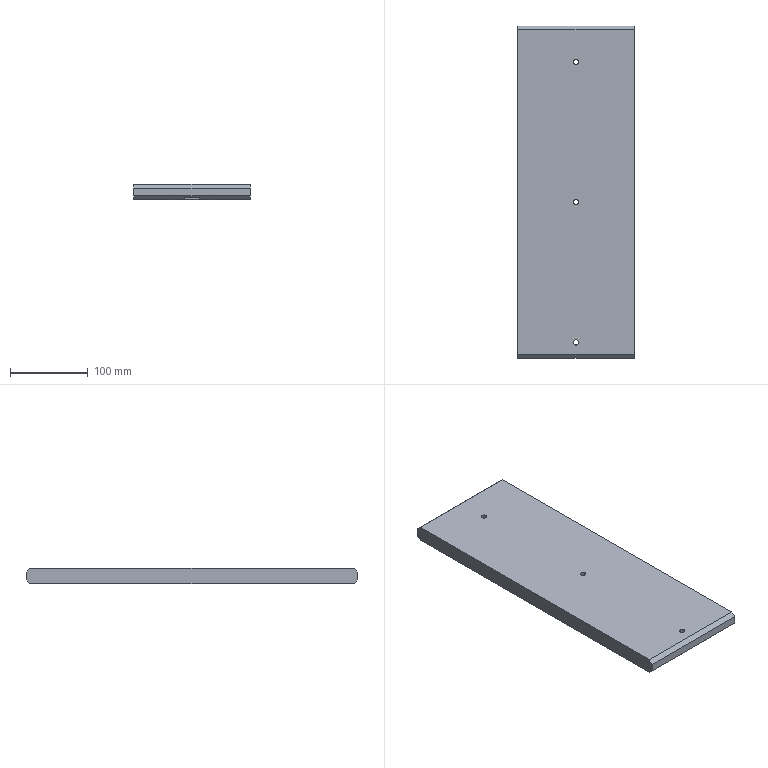Part | SolidWorks | features Chamfer 2, HoleWzd 2, Extrusion 1, ICE 1 | 1 solid | 28 faces | box 150 x 426 x 20 mm | volume 1243356 mm3 | plane 14 | cylinder 10 | cone 4 | commonest cylinder face diameters 6.8 x10
STEP:
#1=CARTESIAN_POINT('',(25.,406.,6.6));
#2=VERTEX_POINT('',#1);
#3=CARTESIAN_POINT('',(25.,406.,13.4));
#4=VERTEX_POINT('',#3);
#5=CARTESIAN_POINT('',(25.,406.,10.));
#6=DIRECTION('',(0.,1.,0.));
#7=DIRECTION('',(0.,0.,1.));
#8=AXIS2_PLACEMENT_3D('',#5,#6,#7);
#9=CIRCLE('',#8,3.4);
#10=EDGE_CURVE('',#2,#4,#9,.T.);
#11=ORIENTED_EDGE('',*,*,#10,.F.);
#12=CARTESIAN_POINT('',(25.,426.,6.6));
#13=VERTEX_POINT('',#12);
#14=CARTESIAN_POINT('',(25.,426.,6.6));
#15=DIRECTION('',(0.,1.,0.));
#16=VECTOR('',#15,1000.);
#17=LINE('',#14,#16);
#18=EDGE_CURVE('',#2,#13,#17,.T.);
#19=ORIENTED_EDGE('',*,*,#18,.T.);
#20=CARTESIAN_POINT('',(25.,426.,13.4));
#21=VERTEX_POINT('',#20);
#22=CARTESIAN_POINT('',(25.,426.,10.));
#23=DIRECTION('',(0.,1.,0.));
#24=DIRECTION('',(0.,0.,1.));
#25=AXIS2_PLACEMENT_3D('',#22,#23,#24);
#26=CIRCLE('',#25,3.4);
#27=EDGE_CURVE('',#13,#21,#26,.T.);
#28=ORIENTED_EDGE('',*,*,#27,.T.);
#29=CARTESIAN_POINT('',(25.,426.,13.4));
#30=DIRECTION('',(0.,1.,0.));
#31=VECTOR('',#30,1000.);
#32=LINE('',#29,#31);
#33=EDGE_CURVE('',#4,#21,#32,.T.);
#34=ORIENTED_EDGE('',*,*,#33,.F.);
#35=EDGE_LOOP('',(#11,#19,#28,#34));
#36=FACE_OUTER_BOUND('',#35,.T.);
#37=CARTESIAN_POINT('',(25.,426.,10.));
#38=DIRECTION('',(0.,1.,0.));
#39=DIRECTION('',(0.,0.,1.));
#40=AXIS2_PLACEMENT_3D('',#37,#38,#39);
#41=CYLINDRICAL_SURFACE('',#40,3.4);
#42=ADVANCED_FACE('',(#36),#41,.F.);
#43=CARTESIAN_POINT('',(25.,403.957,10.));
#44=VERTEX_POINT('',#43);
#45=CARTESIAN_POINT('',(25.,406.,13.4));
#46=DIRECTION('',(0.,0.515,0.8572));
#47=VECTOR('',#46,1000.);
#48=LINE('',#45,#47);
#49=EDGE_CURVE('',#44,#4,#48,.T.);
#50=ORIENTED_EDGE('',*,*,#49,.F.);
#51=CARTESIAN_POINT('',(25.,406.,6.6));
#52=DIRECTION('',(0.,0.515,-0.8572));
#53=VECTOR('',#52,1000.);
#54=LINE('',#51,#53);
#55=EDGE_CURVE('',#44,#2,#54,.T.);
#56=ORIENTED_EDGE('',*,*,#55,.T.);
#57=ORIENTED_EDGE('',*,*,#10,.T.);
#58=EDGE_LOOP('',(#50,#56,#57));
#59=FACE_OUTER_BOUND('',#58,.T.);
#60=CARTESIAN_POINT('',(25.,406.,10.));
#61=DIRECTION('',(0.,1.,0.));
#62=DIRECTION('',(0.,0.,1.));
#63=AXIS2_PLACEMENT_3D('',#60,#61,#62);
#64=CONICAL_SURFACE('',#63,3.4,1.03);
#65=ADVANCED_FACE('',(#59),#64,.F.);
#66=CARTESIAN_POINT('',(125.,406.,6.6));
#67=VERTEX_POINT('',#66);
#68=CARTESIAN_POINT('',(125.,406.,13.4));
#69=VERTEX_POINT('',#68);
#70=CARTESIAN_POINT('',(125.,406.,10.));
#71=DIRECTION('',(0.,1.,0.));
#72=DIRECTION('',(0.,0.,1.));
#73=AXIS2_PLACEMENT_3D('',#70,#71,#72);
#74=CIRCLE('',#73,3.4);
#75=EDGE_CURVE('',#67,#69,#74,.T.);
#76=ORIENTED_EDGE('',*,*,#75,.F.);
#77=CARTESIAN_POINT('',(125.,426.,6.6));
#78=VERTEX_POINT('',#77);
#79=CARTESIAN_POINT('',(125.,426.,6.6));
#80=DIRECTION('',(0.,1.,0.));
#81=VECTOR('',#80,1000.);
#82=LINE('',#79,#81);
#83=EDGE_CURVE('',#67,#78,#82,.T.);
#84=ORIENTED_EDGE('',*,*,#83,.T.);
#85=CARTESIAN_POINT('',(125.,426.,13.4));
#86=VERTEX_POINT('',#85);
#87=CARTESIAN_POINT('',(125.,426.,10.));
#88=DIRECTION('',(0.,1.,0.));
#89=DIRECTION('',(0.,0.,1.));
#90=AXIS2_PLACEMENT_3D('',#87,#88,#89);
#91=CIRCLE('',#90,3.4);
#92=EDGE_CURVE('',#78,#86,#91,.T.);
#93=ORIENTED_EDGE('',*,*,#92,.T.);
#94=CARTESIAN_POINT('',(125.,426.,13.4));
#95=DIRECTION('',(0.,1.,0.));
#96=VECTOR('',#95,1000.);
#97=LINE('',#94,#96);
#98=EDGE_CURVE('',#69,#86,#97,.T.);
#99=ORIENTED_EDGE('',*,*,#98,.F.);
#100=EDGE_LOOP('',(#76,#84,#93,#99));
#101=FACE_OUTER_BOUND('',#100,.T.);
#102=CARTESIAN_POINT('',(125.,426.,10.));
#103=DIRECTION('',(0.,1.,0.));
#104=DIRECTION('',(0.,0.,1.));
#105=AXIS2_PLACEMENT_3D('',#102,#103,#104);
#106=CYLINDRICAL_SURFACE('',#105,3.4);
#107=ADVANCED_FACE('',(#101),#106,.F.);
#108=CARTESIAN_POINT('',(125.,403.957,10.));
#109=VERTEX_POINT('',#108);
#110=CARTESIAN_POINT('',(125.,406.,13.4));
#111=DIRECTION('',(0.,0.515,0.8572));
#112=VECTOR('',#111,1000.);
#113=LINE('',#110,#112);
#114=EDGE_CURVE('',#109,#69,#113,.T.);
#115=ORIENTED_EDGE('',*,*,#114,.F.);
#116=CARTESIAN_POINT('',(125.,406.,6.6));
#117=DIRECTION('',(0.,0.515,-0.8572));
#118=VECTOR('',#117,1000.);
#119=LINE('',#116,#118);
#120=EDGE_CURVE('',#109,#67,#119,.T.);
#121=ORIENTED_EDGE('',*,*,#120,.T.);
#122=ORIENTED_EDGE('',*,*,#75,.T.);
#123=EDGE_LOOP('',(#115,#121,#122));
#124=FACE_OUTER_BOUND('',#123,.T.);
#125=CARTESIAN_POINT('',(125.,406.,10.));
#126=DIRECTION('',(0.,1.,0.));
#127=DIRECTION('',(0.,0.,1.));
#128=AXIS2_PLACEMENT_3D('',#125,#126,#127);
#129=CONICAL_SURFACE('',#128,3.4,1.03);
#130=ADVANCED_FACE('',(#124),#129,.F.);
#131=CARTESIAN_POINT('',(78.4,20.,20.));
#132=VERTEX_POINT('',#131);
#133=CARTESIAN_POINT('',(71.6,20.,20.));
#134=VERTEX_POINT('',#133);
#135=CARTESIAN_POINT('',(75.,20.,20.));
#136=DIRECTION('',(0.,0.,-1.));
#137=DIRECTION('',(-1.,0.,0.));
#138=AXIS2_PLACEMENT_3D('',#135,#136,#137);
#139=CIRCLE('',#138,3.4);
#140=EDGE_CURVE('',#132,#134,#139,.T.);
#141=ORIENTED_EDGE('',*,*,#140,.F.);
#142=CARTESIAN_POINT('',(78.4,20.,3.));
#143=VERTEX_POINT('',#142);
#144=CARTESIAN_POINT('',(78.4,20.,3.));
#145=DIRECTION('',(0.,0.,-1.));
#146=VECTOR('',#145,1000.);
#147=LINE('',#144,#146);
#148=EDGE_CURVE('',#132,#143,#147,.T.);
#149=ORIENTED_EDGE('',*,*,#148,.T.);
#150=CARTESIAN_POINT('',(71.6,20.,3.));
#151=VERTEX_POINT('',#150);
#152=CARTESIAN_POINT('',(75.,20.,3.));
#153=DIRECTION('',(0.,0.,-1.));
#154=DIRECTION('',(-1.,0.,0.));
#155=AXIS2_PLACEMENT_3D('',#152,#153,#154);
#156=CIRCLE('',#155,3.4);
#157=EDGE_CURVE('',#143,#151,#156,.T.);
#158=ORIENTED_EDGE('',*,*,#157,.T.);
#159=CARTESIAN_POINT('',(71.6,20.,3.));
#160=DIRECTION('',(0.,0.,-1.));
#161=VECTOR('',#160,1000.);
#162=LINE('',#159,#161);
#163=EDGE_CURVE('',#134,#151,#162,.T.);
#164=ORIENTED_EDGE('',*,*,#163,.F.);
#165=EDGE_LOOP('',(#141,#149,#158,#164));
#166=FACE_OUTER_BOUND('',#165,.T.);
#167=CARTESIAN_POINT('',(75.,20.,3.));
#168=DIRECTION('',(0.,0.,-1.));
#169=DIRECTION('',(-1.,0.,0.));
#170=AXIS2_PLACEMENT_3D('',#167,#168,#169);
#171=CYLINDRICAL_SURFACE('',#170,3.4);
#172=ADVANCED_FACE('',(#166),#171,.F.);
#173=CARTESIAN_POINT('',(78.4,200.,20.));
#174=VERTEX_POINT('',#173);
#175=CARTESIAN_POINT('',(71.6,200.,20.));
#176=VERTEX_POINT('',#175);
#177=CARTESIAN_POINT('',(75.,200.,20.));
#178=DIRECTION('',(0.,0.,-1.));
#179=DIRECTION('',(-1.,0.,0.));
#180=AXIS2_PLACEMENT_3D('',#177,#178,#179);
#181=CIRCLE('',#180,3.4);
#182=EDGE_CURVE('',#174,#176,#181,.T.);
#183=ORIENTED_EDGE('',*,*,#182,.F.);
#184=CARTESIAN_POINT('',(78.4,200.,3.));
#185=VERTEX_POINT('',#184);
#186=CARTESIAN_POINT('',(78.4,200.,3.));
#187=DIRECTION('',(0.,0.,-1.));
#188=VECTOR('',#187,1000.);
#189=LINE('',#186,#188);
#190=EDGE_CURVE('',#174,#185,#189,.T.);
#191=ORIENTED_EDGE('',*,*,#190,.T.);
#192=CARTESIAN_POINT('',(71.6,200.,3.));
#193=VERTEX_POINT('',#192);
#194=CARTESIAN_POINT('',(75.,200.,3.));
#195=DIRECTION('',(0.,0.,-1.));
#196=DIRECTION('',(-1.,0.,0.));
#197=AXIS2_PLACEMENT_3D('',#194,#195,#196);
#198=CIRCLE('',#197,3.4);
#199=EDGE_CURVE('',#185,#193,#198,.T.);
#200=ORIENTED_EDGE('',*,*,#199,.T.);
#201=CARTESIAN_POINT('',(71.6,200.,3.));
#202=DIRECTION('',(0.,0.,-1.));
#203=VECTOR('',#202,1000.);
#204=LINE('',#201,#203);
#205=EDGE_CURVE('',#176,#193,#204,.T.);
#206=ORIENTED_EDGE('',*,*,#205,.F.);
#207=EDGE_LOOP('',(#183,#191,#200,#206));
#208=FACE_OUTER_BOUND('',#207,.T.);
#209=CARTESIAN_POINT('',(75.,200.,3.));
#210=DIRECTION('',(0.,0.,-1.));
#211=DIRECTION('',(-1.,0.,0.));
#212=AXIS2_PLACEMENT_3D('',#209,#210,#211);
#213=CYLINDRICAL_SURFACE('',#212,3.4);
#214=ADVANCED_FACE('',(#208),#213,.F.);
#215=CARTESIAN_POINT('',(78.4,380.,20.));
#216=VERTEX_POINT('',#215);
#217=CARTESIAN_POINT('',(71.6,380.,20.));
#218=VERTEX_POINT('',#217);
#219=CARTESIAN_POINT('',(75.,380.,20.));
#220=DIRECTION('',(0.,0.,-1.));
#221=DIRECTION('',(-1.,0.,0.));
#222=AXIS2_PLACEMENT_3D('',#219,#220,#221);
#223=CIRCLE('',#222,3.4);
#224=EDGE_CURVE('',#216,#218,#223,.T.);
#225=ORIENTED_EDGE('',*,*,#224,.F.);
#226=CARTESIAN_POINT('',(78.4,380.,3.));
#227=VERTEX_POINT('',#226);
#228=CARTESIAN_POINT('',(78.4,380.,3.));
#229=DIRECTION('',(0.,0.,-1.));
#230=VECTOR('',#229,1000.);
#231=LINE('',#228,#230);
#232=EDGE_CURVE('',#216,#227,#231,.T.);
#233=ORIENTED_EDGE('',*,*,#232,.T.);
#234=CARTESIAN_POINT('',(71.6,380.,3.));
#235=VERTEX_POINT('',#234);
#236=CARTESIAN_POINT('',(75.,380.,3.));
#237=DIRECTION('',(0.,0.,-1.));
#238=DIRECTION('',(-1.,0.,0.));
#239=AXIS2_PLACEMENT_3D('',#236,#237,#238);
#240=CIRCLE('',#239,3.4);
#241=EDGE_CURVE('',#227,#235,#240,.T.);
#242=ORIENTED_EDGE('',*,*,#241,.T.);
#243=CARTESIAN_POINT('',(71.6,380.,3.));
#244=DIRECTION('',(0.,0.,-1.));
#245=VECTOR('',#244,1000.);
#246=LINE('',#243,#245);
#247=EDGE_CURVE('',#218,#235,#246,.T.);
#248=ORIENTED_EDGE('',*,*,#247,.F.);
#249=EDGE_LOOP('',(#225,#233,#242,#248));
#250=FACE_OUTER_BOUND('',#249,.T.);
#251=CARTESIAN_POINT('',(75.,380.,3.));
#252=DIRECTION('',(0.,0.,-1.));
#253=DIRECTION('',(-1.,0.,0.));
#254=AXIS2_PLACEMENT_3D('',#251,#252,#253);
#255=CYLINDRICAL_SURFACE('',#254,3.4);
#256=ADVANCED_FACE('',(#250),#255,.F.);
#257=CARTESIAN_POINT('',(0.,421.,20.));
#258=VERTEX_POINT('',#257);
#259=CARTESIAN_POINT('',(0.,5.,20.));
#260=VERTEX_POINT('',#259);
#261=CARTESIAN_POINT('',(0.,0.,20.));
#262=DIRECTION('',(0.,-1.,0.));
#263=VECTOR('',#262,1000.);
#264=LINE('',#261,#263);
#265=EDGE_CURVE('',#258,#260,#264,.T.);
#266=ORIENTED_EDGE('',*,*,#265,.F.);
#267=CARTESIAN_POINT('',(0.,426.,15.));
#268=VERTEX_POINT('',#267);
#269=CARTESIAN_POINT('',(0.,421.,20.));
#270=DIRECTION('',(0.,0.7071,-0.7071));
#271=VECTOR('',#270,1000.);
#272=LINE('',#269,#271);
#273=EDGE_CURVE('',#258,#268,#272,.T.);
#274=ORIENTED_EDGE('',*,*,#273,.T.);
#275=CARTESIAN_POINT('',(0.,426.,5.));
#276=VERTEX_POINT('',#275);
#277=CARTESIAN_POINT('',(0.,426.,20.));
#278=DIRECTION('',(0.,0.,-1.));
#279=VECTOR('',#278,1000.);
#280=LINE('',#277,#279);
#281=EDGE_CURVE('',#268,#276,#280,.T.);
#282=ORIENTED_EDGE('',*,*,#281,.T.);
#283=CARTESIAN_POINT('',(0.,421.,0.));
#284=VERTEX_POINT('',#283);
#285=CARTESIAN_POINT('',(0.,426.,5.));
#286=DIRECTION('',(0.,-0.7071,-0.7071));
#287=VECTOR('',#286,1000.);
#288=LINE('',#285,#287);
#289=EDGE_CURVE('',#276,#284,#288,.T.);
#290=ORIENTED_EDGE('',*,*,#289,.T.);
#291=CARTESIAN_POINT('',(0.,5.,0.));
#292=VERTEX_POINT('',#291);
#293=CARTESIAN_POINT('',(0.,0.,0.));
#294=DIRECTION('',(0.,-1.,0.));
#295=VECTOR('',#294,1000.);
#296=LINE('',#293,#295);
#297=EDGE_CURVE('',#284,#292,#296,.T.);
#298=ORIENTED_EDGE('',*,*,#297,.T.);
#299=CARTESIAN_POINT('',(0.,0.,5.));
#300=VERTEX_POINT('',#299);
#301=CARTESIAN_POINT('',(0.,0.,5.));
#302=DIRECTION('',(0.,-0.7071,0.7071));
#303=VECTOR('',#302,1000.);
#304=LINE('',#301,#303);
#305=EDGE_CURVE('',#292,#300,#304,.T.);
#306=ORIENTED_EDGE('',*,*,#305,.T.);
#307=CARTESIAN_POINT('',(0.,0.,15.));
#308=VERTEX_POINT('',#307);
#309=CARTESIAN_POINT('',(0.,0.,20.));
#310=DIRECTION('',(0.,0.,-1.));
#311=VECTOR('',#310,1000.);
#312=LINE('',#309,#311);
#313=EDGE_CURVE('',#308,#300,#312,.T.);
#314=ORIENTED_EDGE('',*,*,#313,.F.);
#315=CARTESIAN_POINT('',(0.,5.,20.));
#316=DIRECTION('',(0.,0.7071,0.7071));
#317=VECTOR('',#316,1000.);
#318=LINE('',#315,#317);
#319=EDGE_CURVE('',#308,#260,#318,.T.);
#320=ORIENTED_EDGE('',*,*,#319,.T.);
#321=EDGE_LOOP('',(#266,#274,#282,#290,#298,#306,#314,#320));
#322=FACE_OUTER_BOUND('',#321,.T.);
#323=CARTESIAN_POINT('',(0.,0.,20.));
#324=DIRECTION('',(1.,0.,0.));
#325=DIRECTION('',(0.,0.,-1.));
#326=AXIS2_PLACEMENT_3D('',#323,#324,#325);
#327=PLANE('',#326);
#328=ADVANCED_FACE('',(#322),#327,.F.);
#329=ORIENTED_EDGE('',*,*,#313,.T.);
#330=CARTESIAN_POINT('',(150.,0.,5.));
#331=VERTEX_POINT('',#330);
#332=CARTESIAN_POINT('',(65.,0.,5.));
#333=DIRECTION('',(1.,0.,0.));
#334=VECTOR('',#333,1000.);
#335=LINE('',#332,#334);
#336=EDGE_CURVE('',#300,#331,#335,.T.);
#337=ORIENTED_EDGE('',*,*,#336,.T.);
#338=CARTESIAN_POINT('',(150.,0.,15.));
#339=VERTEX_POINT('',#338);
#340=CARTESIAN_POINT('',(150.,0.,20.));
#341=DIRECTION('',(0.,0.,-1.));
#342=VECTOR('',#341,1000.);
#343=LINE('',#340,#342);
#344=EDGE_CURVE('',#339,#331,#343,.T.);
#345=ORIENTED_EDGE('',*,*,#344,.F.);
#346=CARTESIAN_POINT('',(0.,0.,15.));
#347=DIRECTION('',(-1.,0.,0.));
#348=VECTOR('',#347,1000.);
#349=LINE('',#346,#348);
#350=EDGE_CURVE('',#339,#308,#349,.T.);
#351=ORIENTED_EDGE('',*,*,#350,.T.);
#352=EDGE_LOOP('',(#329,#337,#345,#351));
#353=FACE_OUTER_BOUND('',#352,.T.);
#354=CARTESIAN_POINT('',(0.,0.,20.));
#355=DIRECTION('',(0.,1.,0.));
#356=DIRECTION('',(0.,0.,1.));
#357=AXIS2_PLACEMENT_3D('',#354,#355,#356);
#358=PLANE('',#357);
#359=ADVANCED_FACE('',(#353),#358,.F.);
#360=CARTESIAN_POINT('',(150.,426.,15.));
#361=VERTEX_POINT('',#360);
#362=CARTESIAN_POINT('',(150.,426.,5.));
#363=VERTEX_POINT('',#362);
#364=CARTESIAN_POINT('',(150.,426.,20.));
#365=DIRECTION('',(0.,0.,-1.));
#366=VECTOR('',#365,1000.);
#367=LINE('',#364,#366);
#368=EDGE_CURVE('',#361,#363,#367,.T.);
#369=ORIENTED_EDGE('',*,*,#368,.F.);
#370=CARTESIAN_POINT('',(150.,421.,20.));
#371=VERTEX_POINT('',#370);
#372=CARTESIAN_POINT('',(150.,421.,20.));
#373=DIRECTION('',(0.,-0.7071,0.7071));
#374=VECTOR('',#373,1000.);
#375=LINE('',#372,#374);
#376=EDGE_CURVE('',#361,#371,#375,.T.);
#377=ORIENTED_EDGE('',*,*,#376,.T.);
#378=CARTESIAN_POINT('',(150.,5.,20.));
#379=VERTEX_POINT('',#378);
#380=CARTESIAN_POINT('',(150.,0.,20.));
#381=DIRECTION('',(0.,1.,0.));
#382=VECTOR('',#381,1000.);
#383=LINE('',#380,#382);
#384=EDGE_CURVE('',#379,#371,#383,.T.);
#385=ORIENTED_EDGE('',*,*,#384,.F.);
#386=CARTESIAN_POINT('',(150.,5.,20.));
#387=DIRECTION('',(0.,-0.7071,-0.7071));
#388=VECTOR('',#387,1000.);
#389=LINE('',#386,#388);
#390=EDGE_CURVE('',#379,#339,#389,.T.);
#391=ORIENTED_EDGE('',*,*,#390,.T.);
#392=ORIENTED_EDGE('',*,*,#344,.T.);
#393=CARTESIAN_POINT('',(150.,5.,0.));
#394=VERTEX_POINT('',#393);
#395=CARTESIAN_POINT('',(150.,0.,5.));
#396=DIRECTION('',(0.,0.7071,-0.7071));
#397=VECTOR('',#396,1000.);
#398=LINE('',#395,#397);
#399=EDGE_CURVE('',#331,#394,#398,.T.);
#400=ORIENTED_EDGE('',*,*,#399,.T.);
#401=CARTESIAN_POINT('',(150.,421.,0.));
#402=VERTEX_POINT('',#401);
#403=CARTESIAN_POINT('',(150.,0.,0.));
#404=DIRECTION('',(0.,1.,0.));
#405=VECTOR('',#404,1000.);
#406=LINE('',#403,#405);
#407=EDGE_CURVE('',#394,#402,#406,.T.);
#408=ORIENTED_EDGE('',*,*,#407,.T.);
#409=CARTESIAN_POINT('',(150.,426.,5.));
#410=DIRECTION('',(0.,0.7071,0.7071));
#411=VECTOR('',#410,1000.);
#412=LINE('',#409,#411);
#413=EDGE_CURVE('',#402,#363,#412,.T.);
#414=ORIENTED_EDGE('',*,*,#413,.T.);
#415=EDGE_LOOP('',(#369,#377,#385,#391,#392,#400,#408,#414));
#416=FACE_OUTER_BOUND('',#415,.T.);
#417=CARTESIAN_POINT('',(150.,0.,20.));
#418=DIRECTION('',(-1.,0.,0.));
#419=DIRECTION('',(0.,0.,1.));
#420=AXIS2_PLACEMENT_3D('',#417,#418,#419);
#421=PLANE('',#420);
#422=ADVANCED_FACE('',(#416),#421,.F.);
#423=CARTESIAN_POINT('',(25.,426.,10.));
#424=DIRECTION('',(0.,1.,0.));
#425=DIRECTION('',(0.,0.,1.));
#426=AXIS2_PLACEMENT_3D('',#423,#424,#425);
#427=CIRCLE('',#426,3.4);
#428=EDGE_CURVE('',#21,#13,#427,.T.);
#429=ORIENTED_EDGE('',*,*,#428,.F.);
#430=ORIENTED_EDGE('',*,*,#27,.F.);
#431=EDGE_LOOP('',(#429,#430));
#432=FACE_BOUND('',#431,.T.);
#433=CARTESIAN_POINT('',(125.,426.,10.));
#434=DIRECTION('',(0.,1.,0.));
#435=DIRECTION('',(0.,0.,1.));
#436=AXIS2_PLACEMENT_3D('',#433,#434,#435);
#437=CIRCLE('',#436,3.4);
#438=EDGE_CURVE('',#86,#78,#437,.T.);
#439=ORIENTED_EDGE('',*,*,#438,.F.);
#440=ORIENTED_EDGE('',*,*,#92,.F.);
#441=EDGE_LOOP('',(#439,#440));
#442=FACE_BOUND('',#441,.T.);
#443=ORIENTED_EDGE('',*,*,#281,.F.);
#444=CARTESIAN_POINT('',(0.,426.,15.));
#445=DIRECTION('',(1.,0.,0.));
#446=VECTOR('',#445,1000.);
#447=LINE('',#444,#446);
#448=EDGE_CURVE('',#268,#361,#447,.T.);
#449=ORIENTED_EDGE('',*,*,#448,.T.);
#450=ORIENTED_EDGE('',*,*,#368,.T.);
#451=CARTESIAN_POINT('',(0.,426.,5.));
#452=DIRECTION('',(-1.,0.,0.));
#453=VECTOR('',#452,1000.);
#454=LINE('',#451,#453);
#455=EDGE_CURVE('',#363,#276,#454,.T.);
#456=ORIENTED_EDGE('',*,*,#455,.T.);
#457=EDGE_LOOP('',(#443,#449,#450,#456));
#458=FACE_OUTER_BOUND('',#457,.T.);
#459=CARTESIAN_POINT('',(0.,426.,20.));
#460=DIRECTION('',(0.,-1.,0.));
#461=DIRECTION('',(0.,0.,-1.));
#462=AXIS2_PLACEMENT_3D('',#459,#460,#461);
#463=PLANE('',#462);
#464=ADVANCED_FACE('',(#432,#442,#458),#463,.F.);
#465=CARTESIAN_POINT('',(75.,20.,20.));
#466=DIRECTION('',(0.,0.,-1.));
#467=DIRECTION('',(-1.,0.,0.));
#468=AXIS2_PLACEMENT_3D('',#465,#466,#467);
#469=CIRCLE('',#468,3.4);
#470=EDGE_CURVE('',#134,#132,#469,.T.);
#471=ORIENTED_EDGE('',*,*,#470,.T.);
#472=ORIENTED_EDGE('',*,*,#140,.T.);
#473=EDGE_LOOP('',(#471,#472));
#474=FACE_BOUND('',#473,.T.);
#475=CARTESIAN_POINT('',(75.,200.,20.));
#476=DIRECTION('',(0.,0.,-1.));
#477=DIRECTION('',(-1.,0.,0.));
#478=AXIS2_PLACEMENT_3D('',#475,#476,#477);
#479=CIRCLE('',#478,3.4);
#480=EDGE_CURVE('',#176,#174,#479,.T.);
#481=ORIENTED_EDGE('',*,*,#480,.T.);
#482=ORIENTED_EDGE('',*,*,#182,.T.);
#483=EDGE_LOOP('',(#481,#482));
#484=FACE_BOUND('',#483,.T.);
#485=CARTESIAN_POINT('',(75.,380.,20.));
#486=DIRECTION('',(0.,0.,-1.));
#487=DIRECTION('',(-1.,0.,0.));
#488=AXIS2_PLACEMENT_3D('',#485,#486,#487);
#489=CIRCLE('',#488,3.4);
#490=EDGE_CURVE('',#218,#216,#489,.T.);
#491=ORIENTED_EDGE('',*,*,#490,.T.);
#492=ORIENTED_EDGE('',*,*,#224,.T.);
#493=EDGE_LOOP('',(#491,#492));
#494=FACE_BOUND('',#493,.T.);
#495=ORIENTED_EDGE('',*,*,#384,.T.);
#496=CARTESIAN_POINT('',(0.,421.,20.));
#497=DIRECTION('',(-1.,0.,0.));
#498=VECTOR('',#497,1000.);
#499=LINE('',#496,#498);
#500=EDGE_CURVE('',#371,#258,#499,.T.);
#501=ORIENTED_EDGE('',*,*,#500,.T.);
#502=ORIENTED_EDGE('',*,*,#265,.T.);
#503=CARTESIAN_POINT('',(0.,5.,20.));
#504=DIRECTION('',(1.,0.,0.));
#505=VECTOR('',#504,1000.);
#506=LINE('',#503,#505);
#507=EDGE_CURVE('',#260,#379,#506,.T.);
#508=ORIENTED_EDGE('',*,*,#507,.T.);
#509=EDGE_LOOP('',(#495,#501,#502,#508));
#510=FACE_OUTER_BOUND('',#509,.T.);
#511=CARTESIAN_POINT('',(0.,0.,20.));
#512=DIRECTION('',(0.,0.,-1.));
#513=DIRECTION('',(-1.,0.,0.));
#514=AXIS2_PLACEMENT_3D('',#511,#512,#513);
#515=PLANE('',#514);
#516=ADVANCED_FACE('',(#474,#484,#494,#510),#515,.F.);
#517=ORIENTED_EDGE('',*,*,#297,.F.);
#518=CARTESIAN_POINT('',(150.,421.,0.));
#519=DIRECTION('',(1.,0.,0.));
#520=VECTOR('',#519,1000.);
#521=LINE('',#518,#520);
#522=EDGE_CURVE('',#284,#402,#521,.T.);
#523=ORIENTED_EDGE('',*,*,#522,.T.);
#524=ORIENTED_EDGE('',*,*,#407,.F.);
#525=CARTESIAN_POINT('',(85.,5.,0.));
#526=VERTEX_POINT('',#525);
#527=CARTESIAN_POINT('',(0.,5.,0.));
#528=DIRECTION('',(-1.,0.,0.));
#529=VECTOR('',#528,1000.);
#530=LINE('',#527,#529);
#531=EDGE_CURVE('',#394,#526,#530,.T.);
#532=ORIENTED_EDGE('',*,*,#531,.T.);
#533=CARTESIAN_POINT('',(85.,400.,0.));
#534=VERTEX_POINT('',#533);
#535=CARTESIAN_POINT('',(85.,400.,0.));
#536=DIRECTION('',(0.,-1.,0.));
#537=VECTOR('',#536,1000.);
#538=LINE('',#535,#537);
#539=EDGE_CURVE('',#534,#526,#538,.T.);
#540=ORIENTED_EDGE('',*,*,#539,.F.);
#541=CARTESIAN_POINT('',(65.,400.,0.));
#542=VERTEX_POINT('',#541);
#543=CARTESIAN_POINT('',(85.,400.,0.));
#544=DIRECTION('',(1.,0.,0.));
#545=VECTOR('',#544,1000.);
#546=LINE('',#543,#545);
#547=EDGE_CURVE('',#542,#534,#546,.T.);
#548=ORIENTED_EDGE('',*,*,#547,.F.);
#549=CARTESIAN_POINT('',(65.,5.,0.));
#550=VERTEX_POINT('',#549);
#551=CARTESIAN_POINT('',(65.,400.,0.));
#552=DIRECTION('',(0.,1.,0.));
#553=VECTOR('',#552,1000.);
#554=LINE('',#551,#553);
#555=EDGE_CURVE('',#550,#542,#554,.T.);
#556=ORIENTED_EDGE('',*,*,#555,.F.);
#557=CARTESIAN_POINT('',(0.,5.,0.));
#558=DIRECTION('',(-1.,0.,0.));
#559=VECTOR('',#558,1000.);
#560=LINE('',#557,#559);
#561=EDGE_CURVE('',#550,#292,#560,.T.);
#562=ORIENTED_EDGE('',*,*,#561,.T.);
#563=EDGE_LOOP('',(#517,#523,#524,#532,#540,#548,#556,#562));
#564=FACE_OUTER_BOUND('',#563,.T.);
#565=CARTESIAN_POINT('',(0.,0.,0.));
#566=DIRECTION('',(0.,0.,-1.));
#567=DIRECTION('',(-1.,0.,0.));
#568=AXIS2_PLACEMENT_3D('',#565,#566,#567);
#569=PLANE('',#568);
#570=ADVANCED_FACE('',(#564),#569,.T.);
#571=ORIENTED_EDGE('',*,*,#539,.T.);
#572=CARTESIAN_POINT('',(85.,2.,3.));
#573=VERTEX_POINT('',#572);
#574=CARTESIAN_POINT('',(85.,0.,5.));
#575=DIRECTION('',(0.,-0.7071,0.7071));
#576=VECTOR('',#575,1000.);
#577=LINE('',#574,#576);
#578=EDGE_CURVE('',#526,#573,#577,.T.);
#579=ORIENTED_EDGE('',*,*,#578,.T.);
#580=CARTESIAN_POINT('',(85.,400.,3.));
#581=VERTEX_POINT('',#580);
#582=CARTESIAN_POINT('',(85.,400.,3.));
#583=DIRECTION('',(0.,-1.,0.));
#584=VECTOR('',#583,1000.);
#585=LINE('',#582,#584);
#586=EDGE_CURVE('',#581,#573,#585,.T.);
#587=ORIENTED_EDGE('',*,*,#586,.F.);
#588=CARTESIAN_POINT('',(85.,400.,3.));
#589=DIRECTION('',(0.,0.,-1.));
#590=VECTOR('',#589,1000.);
#591=LINE('',#588,#590);
#592=EDGE_CURVE('',#581,#534,#591,.T.);
#593=ORIENTED_EDGE('',*,*,#592,.T.);
#594=EDGE_LOOP('',(#571,#579,#587,#593));
#595=FACE_OUTER_BOUND('',#594,.T.);
#596=CARTESIAN_POINT('',(85.,400.,3.));
#597=DIRECTION('',(1.,0.,0.));
#598=DIRECTION('',(0.,1.,0.));
#599=AXIS2_PLACEMENT_3D('',#596,#597,#598);
#600=PLANE('',#599);
#601=ADVANCED_FACE('',(#595),#600,.F.);
#602=ORIENTED_EDGE('',*,*,#547,.T.);
#603=ORIENTED_EDGE('',*,*,#592,.F.);
#604=CARTESIAN_POINT('',(65.,400.,3.));
#605=VERTEX_POINT('',#604);
#606=CARTESIAN_POINT('',(85.,400.,3.));
#607=DIRECTION('',(1.,0.,0.));
#608=VECTOR('',#607,1000.);
#609=LINE('',#606,#608);
#610=EDGE_CURVE('',#605,#581,#609,.T.);
#611=ORIENTED_EDGE('',*,*,#610,.F.);
#612=CARTESIAN_POINT('',(65.,400.,3.));
#613=DIRECTION('',(0.,0.,-1.));
#614=VECTOR('',#613,1000.);
#615=LINE('',#612,#614);
#616=EDGE_CURVE('',#605,#542,#615,.T.);
#617=ORIENTED_EDGE('',*,*,#616,.T.);
#618=EDGE_LOOP('',(#602,#603,#611,#617));
#619=FACE_OUTER_BOUND('',#618,.T.);
#620=CARTESIAN_POINT('',(85.,400.,3.));
#621=DIRECTION('',(0.,1.,0.));
#622=DIRECTION('',(0.,0.,1.));
#623=AXIS2_PLACEMENT_3D('',#620,#621,#622);
#624=PLANE('',#623);
#625=ADVANCED_FACE('',(#619),#624,.F.);
#626=CARTESIAN_POINT('',(65.,2.,3.));
#627=VERTEX_POINT('',#626);
#628=CARTESIAN_POINT('',(65.,400.,3.));
#629=DIRECTION('',(0.,1.,0.));
#630=VECTOR('',#629,1000.);
#631=LINE('',#628,#630);
#632=EDGE_CURVE('',#627,#605,#631,.T.);
#633=ORIENTED_EDGE('',*,*,#632,.F.);
#634=CARTESIAN_POINT('',(65.,0.,5.));
#635=DIRECTION('',(0.,0.7071,-0.7071));
#636=VECTOR('',#635,1000.);
#637=LINE('',#634,#636);
#638=EDGE_CURVE('',#627,#550,#637,.T.);
#639=ORIENTED_EDGE('',*,*,#638,.T.);
#640=ORIENTED_EDGE('',*,*,#555,.T.);
#641=ORIENTED_EDGE('',*,*,#616,.F.);
#642=EDGE_LOOP('',(#633,#639,#640,#641));
#643=FACE_OUTER_BOUND('',#642,.T.);
#644=CARTESIAN_POINT('',(65.,400.,3.));
#645=DIRECTION('',(-1.,0.,0.));
#646=DIRECTION('',(0.,-1.,0.));
#647=AXIS2_PLACEMENT_3D('',#644,#645,#646);
#648=PLANE('',#647);
#649=ADVANCED_FACE('',(#643),#648,.F.);
#650=CARTESIAN_POINT('',(75.,20.,3.));
#651=DIRECTION('',(0.,0.,-1.));
#652=DIRECTION('',(-1.,0.,0.));
#653=AXIS2_PLACEMENT_3D('',#650,#651,#652);
#654=CIRCLE('',#653,3.4);
#655=EDGE_CURVE('',#151,#143,#654,.T.);
#656=ORIENTED_EDGE('',*,*,#655,.F.);
#657=ORIENTED_EDGE('',*,*,#157,.F.);
#658=EDGE_LOOP('',(#656,#657));
#659=FACE_BOUND('',#658,.T.);
#660=CARTESIAN_POINT('',(75.,200.,3.));
#661=DIRECTION('',(0.,0.,-1.));
#662=DIRECTION('',(-1.,0.,0.));
#663=AXIS2_PLACEMENT_3D('',#660,#661,#662);
#664=CIRCLE('',#663,3.4);
#665=EDGE_CURVE('',#193,#185,#664,.T.);
#666=ORIENTED_EDGE('',*,*,#665,.F.);
#667=ORIENTED_EDGE('',*,*,#199,.F.);
#668=EDGE_LOOP('',(#666,#667));
#669=FACE_BOUND('',#668,.T.);
#670=CARTESIAN_POINT('',(75.,380.,3.));
#671=DIRECTION('',(0.,0.,-1.));
#672=DIRECTION('',(-1.,0.,0.));
#673=AXIS2_PLACEMENT_3D('',#670,#671,#672);
#674=CIRCLE('',#673,3.4);
#675=EDGE_CURVE('',#235,#227,#674,.T.);
#676=ORIENTED_EDGE('',*,*,#675,.F.);
#677=ORIENTED_EDGE('',*,*,#241,.F.);
#678=EDGE_LOOP('',(#676,#677));
#679=FACE_BOUND('',#678,.T.);
#680=ORIENTED_EDGE('',*,*,#586,.T.);
#681=CARTESIAN_POINT('',(0.,2.,3.));
#682=DIRECTION('',(-1.,0.,0.));
#683=VECTOR('',#682,1000.);
#684=LINE('',#681,#683);
#685=EDGE_CURVE('',#573,#627,#684,.T.);
#686=ORIENTED_EDGE('',*,*,#685,.T.);
#687=ORIENTED_EDGE('',*,*,#632,.T.);
#688=ORIENTED_EDGE('',*,*,#610,.T.);
#689=EDGE_LOOP('',(#680,#686,#687,#688));
#690=FACE_OUTER_BOUND('',#689,.T.);
#691=CARTESIAN_POINT('',(0.,0.,3.));
#692=DIRECTION('',(0.,0.,-1.));
#693=DIRECTION('',(-1.,0.,0.));
#694=AXIS2_PLACEMENT_3D('',#691,#692,#693);
#695=PLANE('',#694);
#696=ADVANCED_FACE('',(#659,#669,#679,#690),#695,.T.);
#697=ORIENTED_EDGE('',*,*,#232,.F.);
#698=ORIENTED_EDGE('',*,*,#490,.F.);
#699=ORIENTED_EDGE('',*,*,#247,.T.);
#700=ORIENTED_EDGE('',*,*,#675,.T.);
#701=EDGE_LOOP('',(#697,#698,#699,#700));
#702=FACE_OUTER_BOUND('',#701,.T.);
#703=CARTESIAN_POINT('',(75.,380.,3.));
#704=DIRECTION('',(0.,0.,-1.));
#705=DIRECTION('',(-1.,0.,0.));
#706=AXIS2_PLACEMENT_3D('',#703,#704,#705);
#707=CYLINDRICAL_SURFACE('',#706,3.4);
#708=ADVANCED_FACE('',(#702),#707,.F.);
#709=ORIENTED_EDGE('',*,*,#190,.F.);
#710=ORIENTED_EDGE('',*,*,#480,.F.);
#711=ORIENTED_EDGE('',*,*,#205,.T.);
#712=ORIENTED_EDGE('',*,*,#665,.T.);
#713=EDGE_LOOP('',(#709,#710,#711,#712));
#714=FACE_OUTER_BOUND('',#713,.T.);
#715=CARTESIAN_POINT('',(75.,200.,3.));
#716=DIRECTION('',(0.,0.,-1.));
#717=DIRECTION('',(-1.,0.,0.));
#718=AXIS2_PLACEMENT_3D('',#715,#716,#717);
#719=CYLINDRICAL_SURFACE('',#718,3.4);
#720=ADVANCED_FACE('',(#714),#719,.F.);
#721=ORIENTED_EDGE('',*,*,#148,.F.);
#722=ORIENTED_EDGE('',*,*,#470,.F.);
#723=ORIENTED_EDGE('',*,*,#163,.T.);
#724=ORIENTED_EDGE('',*,*,#655,.T.);
#725=EDGE_LOOP('',(#721,#722,#723,#724));
#726=FACE_OUTER_BOUND('',#725,.T.);
#727=CARTESIAN_POINT('',(75.,20.,3.));
#728=DIRECTION('',(0.,0.,-1.));
#729=DIRECTION('',(-1.,0.,0.));
#730=AXIS2_PLACEMENT_3D('',#727,#728,#729);
#731=CYLINDRICAL_SURFACE('',#730,3.4);
#732=ADVANCED_FACE('',(#726),#731,.F.);
#733=ORIENTED_EDGE('',*,*,#120,.F.);
#734=ORIENTED_EDGE('',*,*,#114,.T.);
#735=CARTESIAN_POINT('',(125.,406.,10.));
#736=DIRECTION('',(0.,1.,0.));
#737=DIRECTION('',(0.,0.,1.));
#738=AXIS2_PLACEMENT_3D('',#735,#736,#737);
#739=CIRCLE('',#738,3.4);
#740=EDGE_CURVE('',#69,#67,#739,.T.);
#741=ORIENTED_EDGE('',*,*,#740,.T.);
#742=EDGE_LOOP('',(#733,#734,#741));
#743=FACE_OUTER_BOUND('',#742,.T.);
#744=CARTESIAN_POINT('',(125.,406.,10.));
#745=DIRECTION('',(0.,1.,0.));
#746=DIRECTION('',(0.,0.,1.));
#747=AXIS2_PLACEMENT_3D('',#744,#745,#746);
#748=CONICAL_SURFACE('',#747,3.4,1.03);
#749=ADVANCED_FACE('',(#743),#748,.F.);
#750=ORIENTED_EDGE('',*,*,#83,.F.);
#751=ORIENTED_EDGE('',*,*,#740,.F.);
#752=ORIENTED_EDGE('',*,*,#98,.T.);
#753=ORIENTED_EDGE('',*,*,#438,.T.);
#754=EDGE_LOOP('',(#750,#751,#752,#753));
#755=FACE_OUTER_BOUND('',#754,.T.);
#756=CARTESIAN_POINT('',(125.,426.,10.));
#757=DIRECTION('',(0.,1.,0.));
#758=DIRECTION('',(0.,0.,1.));
#759=AXIS2_PLACEMENT_3D('',#756,#757,#758);
#760=CYLINDRICAL_SURFACE('',#759,3.4);
#761=ADVANCED_FACE('',(#755),#760,.F.);
#762=ORIENTED_EDGE('',*,*,#55,.F.);
#763=ORIENTED_EDGE('',*,*,#49,.T.);
#764=CARTESIAN_POINT('',(25.,406.,10.));
#765=DIRECTION('',(0.,1.,0.));
#766=DIRECTION('',(0.,0.,1.));
#767=AXIS2_PLACEMENT_3D('',#764,#765,#766);
#768=CIRCLE('',#767,3.4);
#769=EDGE_CURVE('',#4,#2,#768,.T.);
#770=ORIENTED_EDGE('',*,*,#769,.T.);
#771=EDGE_LOOP('',(#762,#763,#770));
#772=FACE_OUTER_BOUND('',#771,.T.);
#773=CARTESIAN_POINT('',(25.,406.,10.));
#774=DIRECTION('',(0.,1.,0.));
#775=DIRECTION('',(0.,0.,1.));
#776=AXIS2_PLACEMENT_3D('',#773,#774,#775);
#777=CONICAL_SURFACE('',#776,3.4,1.03);
#778=ADVANCED_FACE('',(#772),#777,.F.);
#779=ORIENTED_EDGE('',*,*,#18,.F.);
#780=ORIENTED_EDGE('',*,*,#769,.F.);
#781=ORIENTED_EDGE('',*,*,#33,.T.);
#782=ORIENTED_EDGE('',*,*,#428,.T.);
#783=EDGE_LOOP('',(#779,#780,#781,#782));
#784=FACE_OUTER_BOUND('',#783,.T.);
#785=CARTESIAN_POINT('',(25.,426.,10.));
#786=DIRECTION('',(0.,1.,0.));
#787=DIRECTION('',(0.,0.,1.));
#788=AXIS2_PLACEMENT_3D('',#785,#786,#787);
#789=CYLINDRICAL_SURFACE('',#788,3.4);
#790=ADVANCED_FACE('',(#784),#789,.F.);
#791=ORIENTED_EDGE('',*,*,#305,.F.);
#792=ORIENTED_EDGE('',*,*,#561,.F.);
#793=ORIENTED_EDGE('',*,*,#638,.F.);
#794=ORIENTED_EDGE('',*,*,#685,.F.);
#795=ORIENTED_EDGE('',*,*,#578,.F.);
#796=ORIENTED_EDGE('',*,*,#531,.F.);
#797=ORIENTED_EDGE('',*,*,#399,.F.);
#798=ORIENTED_EDGE('',*,*,#336,.F.);
#799=EDGE_LOOP('',(#791,#792,#793,#794,#795,#796,#797,#798));
#800=FACE_OUTER_BOUND('',#799,.T.);
#801=CARTESIAN_POINT('',(0.,0.,5.));
#802=DIRECTION('',(0.,-0.7071,-0.7071));
#803=DIRECTION('',(-1.,0.,0.));
#804=AXIS2_PLACEMENT_3D('',#801,#802,#803);
#805=PLANE('',#804);
#806=ADVANCED_FACE('',(#800),#805,.T.);
#807=ORIENTED_EDGE('',*,*,#319,.F.);
#808=ORIENTED_EDGE('',*,*,#350,.F.);
#809=ORIENTED_EDGE('',*,*,#390,.F.);
#810=ORIENTED_EDGE('',*,*,#507,.F.);
#811=EDGE_LOOP('',(#807,#808,#809,#810));
#812=FACE_OUTER_BOUND('',#811,.T.);
#813=CARTESIAN_POINT('',(0.,5.,20.));
#814=DIRECTION('',(0.,0.7071,-0.7071));
#815=DIRECTION('',(1.,0.,0.));
#816=AXIS2_PLACEMENT_3D('',#813,#814,#815);
#817=PLANE('',#816);
#818=ADVANCED_FACE('',(#812),#817,.F.);
#819=ORIENTED_EDGE('',*,*,#376,.F.);
#820=ORIENTED_EDGE('',*,*,#448,.F.);
#821=ORIENTED_EDGE('',*,*,#273,.F.);
#822=ORIENTED_EDGE('',*,*,#500,.F.);
#823=EDGE_LOOP('',(#819,#820,#821,#822));
#824=FACE_OUTER_BOUND('',#823,.T.);
#825=CARTESIAN_POINT('',(0.,421.,20.));
#826=DIRECTION('',(0.,-0.7071,-0.7071));
#827=DIRECTION('',(-1.,0.,0.));
#828=AXIS2_PLACEMENT_3D('',#825,#826,#827);
#829=PLANE('',#828);
#830=ADVANCED_FACE('',(#824),#829,.F.);
#831=ORIENTED_EDGE('',*,*,#413,.F.);
#832=ORIENTED_EDGE('',*,*,#522,.F.);
#833=ORIENTED_EDGE('',*,*,#289,.F.);
#834=ORIENTED_EDGE('',*,*,#455,.F.);
#835=EDGE_LOOP('',(#831,#832,#833,#834));
#836=FACE_OUTER_BOUND('',#835,.T.);
#837=CARTESIAN_POINT('',(0.,426.,5.));
#838=DIRECTION('',(0.,0.7071,-0.7071));
#839=DIRECTION('',(1.,0.,0.));
#840=AXIS2_PLACEMENT_3D('',#837,#838,#839);
#841=PLANE('',#840);
#842=ADVANCED_FACE('',(#836),#841,.T.);
#843=CLOSED_SHELL('',(#42,#65,#107,#130,#172,#214,#256,#328,#359,#422,#464,#516,#570,#601,#625,#649,#696,#708,#720,#732,#749,#761,#778,#790,#806,#818,#830,#842));
#844=MANIFOLD_SOLID_BREP('',#843);
#845=CARTESIAN_POINT('',(0.,0.,0.));
#846=DIRECTION('',(0.,0.,1.));
#847=DIRECTION('',(1.,0.,0.));
#848=AXIS2_PLACEMENT_3D('',#845,#846,#847);
#849=(LENGTH_UNIT()NAMED_UNIT(*)SI_UNIT(.MILLI.,.METRE.));
#850=UNCERTAINTY_MEASURE_WITH_UNIT(LENGTH_MEASURE(0.00001),#849,'','');
#851=(NAMED_UNIT(*)PLANE_ANGLE_UNIT()SI_UNIT($,.RADIAN.));
#852=(NAMED_UNIT(*)SI_UNIT($,.STERADIAN.)SOLID_ANGLE_UNIT());
#853=(GEOMETRIC_REPRESENTATION_CONTEXT(3)GLOBAL_UNCERTAINTY_ASSIGNED_CONTEXT((#850))GLOBAL_UNIT_ASSIGNED_CONTEXT((#849,#851,#852))REPRESENTATION_CONTEXT('',''));
#854=ADVANCED_BREP_SHAPE_REPRESENTATION('',(#844,#848),#853);